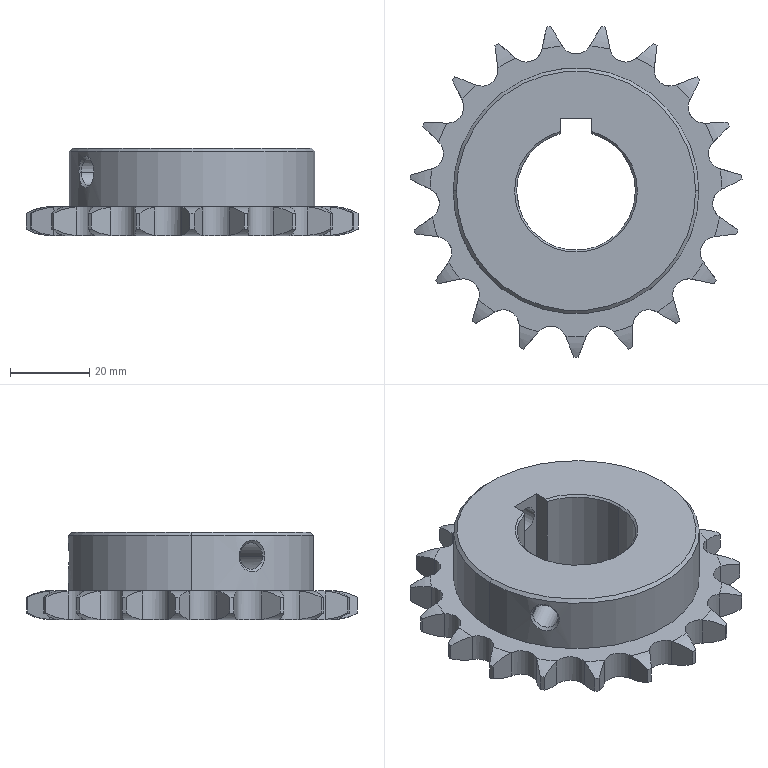Part | SolidWorks | features MBimport 1 | 1 solid | 130 faces | box 83.793 x 83.51 x 22.064 mm | volume 58564 mm3 | cylinder 53 | plane 44 | torus 21 | cone 12 | commonest cylinder face diameters 8.04 x25 84 x19 6.647 x4 30 x3 62 x2